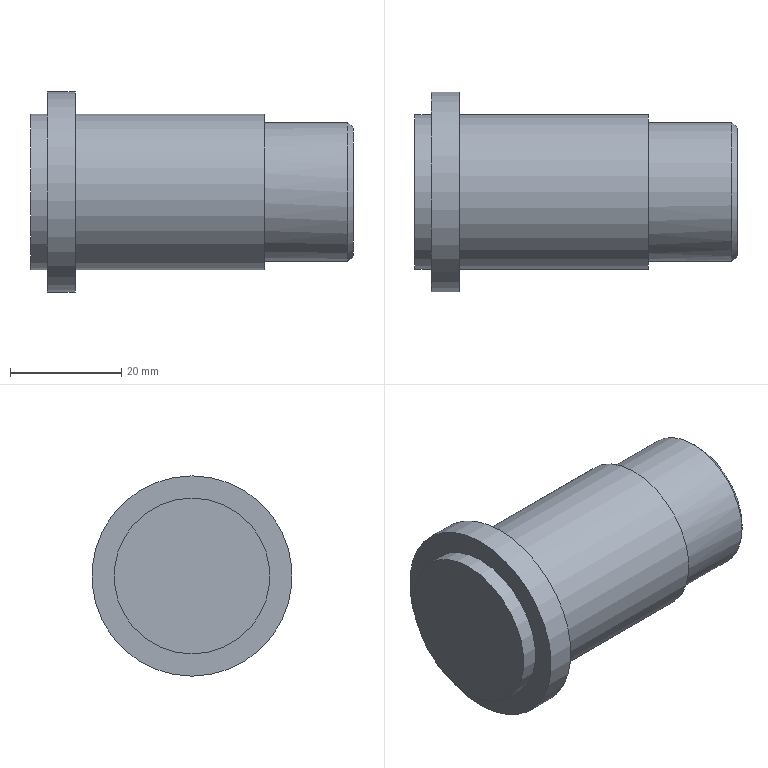Part | STEP file | zhou2 | 1 solid | 12 faces | box 58 x 36 x 36 mm | volume 34937 mm3 | cylinder 5 | plane 5 | cone 2 | commonest cylinder face diameters 28 x2 6.8 x1 25 x1 36 x1
STEP:
#1=CARTESIAN_POINT('',(0.,0.,0.));
#2=DIRECTION('',(0.,0.,1.));
#3=DIRECTION('',(1.,0.,0.));
#4=AXIS2_PLACEMENT_3D('',#1,#2,#3);
#5=CARTESIAN_POINT('',(8.,0.,14.));
#6=VERTEX_POINT('',#5);
#7=CARTESIAN_POINT('',(8.,0.,0.));
#8=DIRECTION('',(1.,0.,0.));
#9=DIRECTION('',(0.,0.,1.));
#10=AXIS2_PLACEMENT_3D('',#7,#8,#9);
#11=CIRCLE('',#10,14.);
#12=CARTESIAN_POINT('',(0.,0.,0.));
#13=DIRECTION('',(-1.,0.,0.));
#14=DIRECTION('',(0.,0.,1.));
#15=AXIS2_PLACEMENT_3D('',#12,#13,#14);
#16=CYLINDRICAL_SURFACE('',#15,14.);
#17=CARTESIAN_POINT('',(6.283,-8.));
#18=DIRECTION('',(-1.,0.));
#19=VECTOR('',#18,1.);
#20=LINE('',#17,#19);
#21=(GEOMETRIC_REPRESENTATION_CONTEXT(2)PARAMETRIC_REPRESENTATION_CONTEXT()REPRESENTATION_CONTEXT('',''));
#22=DEFINITIONAL_REPRESENTATION('',(#20),#21);
#23=PCURVE('',#16,#22);
#24=CARTESIAN_POINT('',(8.,18.,0.));
#25=DIRECTION('',(-1.,0.,0.));
#26=DIRECTION('',(0.,0.,1.));
#27=AXIS2_PLACEMENT_3D('',#24,#25,#26);
#28=PLANE('',#27);
#29=CARTESIAN_POINT('',(14.,-18.));
#30=CARTESIAN_POINT('',(14.,-42.249));
#31=CARTESIAN_POINT('',(-7.,-30.124));
#32=CARTESIAN_POINT('',(-28.,-18.));
#33=CARTESIAN_POINT('',(-7.,-5.876));
#34=CARTESIAN_POINT('',(14.,6.249));
#35=CARTESIAN_POINT('',(14.,-18.));
#36=(BOUNDED_CURVE()B_SPLINE_CURVE(2,(#29,#30,#31,#32,#33,#34,#35),.UNSPECIFIED.,.T.,.F.)B_SPLINE_CURVE_WITH_KNOTS((1,2,2,2,2,1),(-2.094,0.,2.094,4.189,6.283,8.378),.UNSPECIFIED.)CURVE()GEOMETRIC_REPRESENTATION_ITEM()RATIONAL_B_SPLINE_CURVE((1.,0.5,1.,0.5,1.,0.5,1.))REPRESENTATION_ITEM(''));
#37=(GEOMETRIC_REPRESENTATION_CONTEXT(2)PARAMETRIC_REPRESENTATION_CONTEXT()REPRESENTATION_CONTEXT('',''));
#38=DEFINITIONAL_REPRESENTATION('',(#36),#37);
#39=PCURVE('',#28,#38);
#40=SURFACE_CURVE('',#11,(#23,#39),.PCURVE_S1.);
#41=EDGE_CURVE('',#6,#6,#40,.T.);
#42=ORIENTED_EDGE('',*,*,#41,.T.);
#43=CARTESIAN_POINT('',(42.,0.,14.));
#44=VERTEX_POINT('',#43);
#45=CARTESIAN_POINT('',(42.,0.,14.));
#46=CARTESIAN_POINT('',(8.,0.,14.));
#47=B_SPLINE_CURVE_WITH_KNOTS('',1,(#45,#46),.UNSPECIFIED.,.F.,.F.,(2,2),(-42.,-8.),.PIECEWISE_BEZIER_KNOTS.);
#48=CARTESIAN_POINT('',(0.,0.));
#49=DIRECTION('',(0.,1.));
#50=VECTOR('',#49,1.);
#51=LINE('',#48,#50);
#52=(GEOMETRIC_REPRESENTATION_CONTEXT(2)PARAMETRIC_REPRESENTATION_CONTEXT()REPRESENTATION_CONTEXT('',''));
#53=DEFINITIONAL_REPRESENTATION('',(#51),#52);
#54=PCURVE('',#16,#53);
#55=CARTESIAN_POINT('',(6.283,0.));
#56=DIRECTION('',(0.,1.));
#57=VECTOR('',#56,1.);
#58=LINE('',#55,#57);
#59=(GEOMETRIC_REPRESENTATION_CONTEXT(2)PARAMETRIC_REPRESENTATION_CONTEXT()REPRESENTATION_CONTEXT('',''));
#60=DEFINITIONAL_REPRESENTATION('',(#58),#59);
#61=PCURVE('',#16,#60);
#62=SEAM_CURVE('',#47,(#54,#61),.PCURVE_S1.);
#63=EDGE_CURVE('',#44,#6,#62,.T.);
#64=ORIENTED_EDGE('',*,*,#63,.F.);
#65=CARTESIAN_POINT('',(42.,0.,0.));
#66=DIRECTION('',(-1.,0.,0.));
#67=DIRECTION('',(0.,0.,1.));
#68=AXIS2_PLACEMENT_3D('',#65,#66,#67);
#69=CIRCLE('',#68,14.);
#70=CARTESIAN_POINT('',(0.,-42.));
#71=DIRECTION('',(1.,0.));
#72=VECTOR('',#71,1.);
#73=LINE('',#70,#72);
#74=(GEOMETRIC_REPRESENTATION_CONTEXT(2)PARAMETRIC_REPRESENTATION_CONTEXT()REPRESENTATION_CONTEXT('',''));
#75=DEFINITIONAL_REPRESENTATION('',(#73),#74);
#76=PCURVE('',#16,#75);
#77=CARTESIAN_POINT('',(42.,14.,0.));
#78=DIRECTION('',(-1.,0.,0.));
#79=DIRECTION('',(0.,0.,1.));
#80=AXIS2_PLACEMENT_3D('',#77,#78,#79);
#81=PLANE('',#80);
#82=CARTESIAN_POINT('',(0.,-14.));
#83=DIRECTION('',(1.,0.));
#84=AXIS2_PLACEMENT_2D('',#82,#83);
#85=CIRCLE('',#84,14.);
#86=(GEOMETRIC_REPRESENTATION_CONTEXT(2)PARAMETRIC_REPRESENTATION_CONTEXT()REPRESENTATION_CONTEXT('',''));
#87=DEFINITIONAL_REPRESENTATION('',(#85),#86);
#88=PCURVE('',#81,#87);
#89=SURFACE_CURVE('',#69,(#76,#88),.PCURVE_S1.);
#90=EDGE_CURVE('',#44,#44,#89,.T.);
#91=ORIENTED_EDGE('',*,*,#90,.T.);
#92=ORIENTED_EDGE('',*,*,#63,.T.);
#93=EDGE_LOOP('',(#42,#64,#91,#92));
#94=FACE_BOUND('',#93,.T.);
#95=ADVANCED_FACE('',(#94),#16,.T.);
#96=ORIENTED_EDGE('',*,*,#41,.F.);
#97=EDGE_LOOP('',(#96));
#98=FACE_BOUND('',#97,.T.);
#99=CARTESIAN_POINT('',(8.,0.,18.));
#100=VERTEX_POINT('',#99);
#101=CARTESIAN_POINT('',(8.,0.,0.));
#102=DIRECTION('',(-1.,0.,0.));
#103=DIRECTION('',(0.,0.,1.));
#104=AXIS2_PLACEMENT_3D('',#101,#102,#103);
#105=CIRCLE('',#104,18.);
#106=CARTESIAN_POINT('',(0.,-18.));
#107=DIRECTION('',(1.,0.));
#108=AXIS2_PLACEMENT_2D('',#106,#107);
#109=CIRCLE('',#108,18.);
#110=(GEOMETRIC_REPRESENTATION_CONTEXT(2)PARAMETRIC_REPRESENTATION_CONTEXT()REPRESENTATION_CONTEXT('',''));
#111=DEFINITIONAL_REPRESENTATION('',(#109),#110);
#112=PCURVE('',#28,#111);
#113=CARTESIAN_POINT('',(0.,0.,0.));
#114=DIRECTION('',(-1.,0.,0.));
#115=DIRECTION('',(0.,0.,1.));
#116=AXIS2_PLACEMENT_3D('',#113,#114,#115);
#117=CYLINDRICAL_SURFACE('',#116,18.);
#118=CARTESIAN_POINT('',(0.,-8.));
#119=DIRECTION('',(1.,0.));
#120=VECTOR('',#119,1.);
#121=LINE('',#118,#120);
#122=(GEOMETRIC_REPRESENTATION_CONTEXT(2)PARAMETRIC_REPRESENTATION_CONTEXT()REPRESENTATION_CONTEXT('',''));
#123=DEFINITIONAL_REPRESENTATION('',(#121),#122);
#124=PCURVE('',#117,#123);
#125=SURFACE_CURVE('',#105,(#112,#124),.PCURVE_S1.);
#126=EDGE_CURVE('',#100,#100,#125,.T.);
#127=ORIENTED_EDGE('',*,*,#126,.F.);
#128=EDGE_LOOP('',(#127));
#129=FACE_BOUND('',#128,.T.);
#130=ADVANCED_FACE('',(#98,#129),#28,.F.);
#131=CARTESIAN_POINT('',(42.,0.,12.5));
#132=VERTEX_POINT('',#131);
#133=CARTESIAN_POINT('',(42.,0.,0.));
#134=DIRECTION('',(1.,0.,0.));
#135=DIRECTION('',(0.,0.,1.));
#136=AXIS2_PLACEMENT_3D('',#133,#134,#135);
#137=CIRCLE('',#136,12.5);
#138=CARTESIAN_POINT('',(12.5,-14.));
#139=CARTESIAN_POINT('',(12.5,-35.651));
#140=CARTESIAN_POINT('',(-6.25,-24.825));
#141=CARTESIAN_POINT('',(-25.,-14.));
#142=CARTESIAN_POINT('',(-6.25,-3.175));
#143=CARTESIAN_POINT('',(12.5,7.651));
#144=CARTESIAN_POINT('',(12.5,-14.));
#145=(BOUNDED_CURVE()B_SPLINE_CURVE(2,(#138,#139,#140,#141,#142,#143,#144),.UNSPECIFIED.,.T.,.F.)B_SPLINE_CURVE_WITH_KNOTS((1,2,2,2,2,1),(-2.094,0.,2.094,4.189,6.283,8.378),.UNSPECIFIED.)CURVE()GEOMETRIC_REPRESENTATION_ITEM()RATIONAL_B_SPLINE_CURVE((1.,0.5,1.,0.5,1.,0.5,1.))REPRESENTATION_ITEM(''));
#146=(GEOMETRIC_REPRESENTATION_CONTEXT(2)PARAMETRIC_REPRESENTATION_CONTEXT()REPRESENTATION_CONTEXT('',''));
#147=DEFINITIONAL_REPRESENTATION('',(#145),#146);
#148=PCURVE('',#81,#147);
#149=CARTESIAN_POINT('',(0.,0.,0.));
#150=DIRECTION('',(-1.,0.,0.));
#151=DIRECTION('',(0.,0.,1.));
#152=AXIS2_PLACEMENT_3D('',#149,#150,#151);
#153=CYLINDRICAL_SURFACE('',#152,12.5);
#154=CARTESIAN_POINT('',(6.283,-42.));
#155=DIRECTION('',(-1.,0.));
#156=VECTOR('',#155,1.);
#157=LINE('',#154,#156);
#158=(GEOMETRIC_REPRESENTATION_CONTEXT(2)PARAMETRIC_REPRESENTATION_CONTEXT()REPRESENTATION_CONTEXT('',''));
#159=DEFINITIONAL_REPRESENTATION('',(#157),#158);
#160=PCURVE('',#153,#159);
#161=SURFACE_CURVE('',#137,(#148,#160),.PCURVE_S1.);
#162=EDGE_CURVE('',#132,#132,#161,.T.);
#163=ORIENTED_EDGE('',*,*,#162,.F.);
#164=EDGE_LOOP('',(#163));
#165=FACE_BOUND('',#164,.T.);
#166=ORIENTED_EDGE('',*,*,#90,.F.);
#167=EDGE_LOOP('',(#166));
#168=FACE_BOUND('',#167,.T.);
#169=ADVANCED_FACE('',(#165,#168),#81,.F.);
#170=CARTESIAN_POINT('',(3.,0.,18.));
#171=VERTEX_POINT('',#170);
#172=CARTESIAN_POINT('',(3.,0.,0.));
#173=DIRECTION('',(1.,0.,0.));
#174=DIRECTION('',(0.,0.,1.));
#175=AXIS2_PLACEMENT_3D('',#172,#173,#174);
#176=CIRCLE('',#175,18.);
#177=CARTESIAN_POINT('',(6.283,-3.));
#178=DIRECTION('',(-1.,0.));
#179=VECTOR('',#178,1.);
#180=LINE('',#177,#179);
#181=(GEOMETRIC_REPRESENTATION_CONTEXT(2)PARAMETRIC_REPRESENTATION_CONTEXT()REPRESENTATION_CONTEXT('',''));
#182=DEFINITIONAL_REPRESENTATION('',(#180),#181);
#183=PCURVE('',#117,#182);
#184=CARTESIAN_POINT('',(3.,14.,0.));
#185=DIRECTION('',(1.,0.,0.));
#186=DIRECTION('',(0.,0.,-1.));
#187=AXIS2_PLACEMENT_3D('',#184,#185,#186);
#188=PLANE('',#187);
#189=CARTESIAN_POINT('',(0.,-14.));
#190=DIRECTION('',(-1.,0.));
#191=AXIS2_PLACEMENT_2D('',#189,#190);
#192=CIRCLE('',#191,18.);
#193=(GEOMETRIC_REPRESENTATION_CONTEXT(2)PARAMETRIC_REPRESENTATION_CONTEXT()REPRESENTATION_CONTEXT('',''));
#194=DEFINITIONAL_REPRESENTATION('',(#192),#193);
#195=PCURVE('',#188,#194);
#196=SURFACE_CURVE('',#176,(#183,#195),.PCURVE_S1.);
#197=EDGE_CURVE('',#171,#171,#196,.T.);
#198=ORIENTED_EDGE('',*,*,#197,.T.);
#199=CARTESIAN_POINT('',(8.,0.,18.));
#200=CARTESIAN_POINT('',(3.,0.,18.));
#201=B_SPLINE_CURVE_WITH_KNOTS('',1,(#199,#200),.UNSPECIFIED.,.F.,.F.,(2,2),(-8.,-3.),.PIECEWISE_BEZIER_KNOTS.);
#202=CARTESIAN_POINT('',(0.,0.));
#203=DIRECTION('',(0.,1.));
#204=VECTOR('',#203,1.);
#205=LINE('',#202,#204);
#206=(GEOMETRIC_REPRESENTATION_CONTEXT(2)PARAMETRIC_REPRESENTATION_CONTEXT()REPRESENTATION_CONTEXT('',''));
#207=DEFINITIONAL_REPRESENTATION('',(#205),#206);
#208=PCURVE('',#117,#207);
#209=CARTESIAN_POINT('',(6.283,0.));
#210=DIRECTION('',(0.,1.));
#211=VECTOR('',#210,1.);
#212=LINE('',#209,#211);
#213=(GEOMETRIC_REPRESENTATION_CONTEXT(2)PARAMETRIC_REPRESENTATION_CONTEXT()REPRESENTATION_CONTEXT('',''));
#214=DEFINITIONAL_REPRESENTATION('',(#212),#213);
#215=PCURVE('',#117,#214);
#216=SEAM_CURVE('',#201,(#208,#215),.PCURVE_S1.);
#217=EDGE_CURVE('',#100,#171,#216,.T.);
#218=ORIENTED_EDGE('',*,*,#217,.F.);
#219=ORIENTED_EDGE('',*,*,#126,.T.);
#220=ORIENTED_EDGE('',*,*,#217,.T.);
#221=EDGE_LOOP('',(#198,#218,#219,#220));
#222=FACE_BOUND('',#221,.T.);
#223=ADVANCED_FACE('',(#222),#117,.T.);
#224=ORIENTED_EDGE('',*,*,#162,.T.);
#225=CARTESIAN_POINT('',(57.,0.,12.5));
#226=VERTEX_POINT('',#225);
#227=CARTESIAN_POINT('',(57.,0.,12.5));
#228=CARTESIAN_POINT('',(42.,0.,12.5));
#229=B_SPLINE_CURVE_WITH_KNOTS('',1,(#227,#228),.UNSPECIFIED.,.F.,.F.,(2,2),(-57.,-42.),.PIECEWISE_BEZIER_KNOTS.);
#230=CARTESIAN_POINT('',(0.,0.));
#231=DIRECTION('',(0.,1.));
#232=VECTOR('',#231,1.);
#233=LINE('',#230,#232);
#234=(GEOMETRIC_REPRESENTATION_CONTEXT(2)PARAMETRIC_REPRESENTATION_CONTEXT()REPRESENTATION_CONTEXT('',''));
#235=DEFINITIONAL_REPRESENTATION('',(#233),#234);
#236=PCURVE('',#153,#235);
#237=CARTESIAN_POINT('',(6.283,0.));
#238=DIRECTION('',(0.,1.));
#239=VECTOR('',#238,1.);
#240=LINE('',#237,#239);
#241=(GEOMETRIC_REPRESENTATION_CONTEXT(2)PARAMETRIC_REPRESENTATION_CONTEXT()REPRESENTATION_CONTEXT('',''));
#242=DEFINITIONAL_REPRESENTATION('',(#240),#241);
#243=PCURVE('',#153,#242);
#244=SEAM_CURVE('',#229,(#236,#243),.PCURVE_S1.);
#245=EDGE_CURVE('',#226,#132,#244,.T.);
#246=ORIENTED_EDGE('',*,*,#245,.F.);
#247=CARTESIAN_POINT('',(57.,-12.5,0.));
#248=VERTEX_POINT('',#247);
#249=CARTESIAN_POINT('',(57.,0.,0.));
#250=DIRECTION('',(-1.,0.,0.));
#251=DIRECTION('',(0.,0.,1.));
#252=AXIS2_PLACEMENT_3D('',#249,#250,#251);
#253=CIRCLE('',#252,12.5);
#254=CARTESIAN_POINT('',(0.,-57.));
#255=DIRECTION('',(1.,0.));
#256=VECTOR('',#255,1.);
#257=LINE('',#254,#256);
#258=(GEOMETRIC_REPRESENTATION_CONTEXT(2)PARAMETRIC_REPRESENTATION_CONTEXT()REPRESENTATION_CONTEXT('',''));
#259=DEFINITIONAL_REPRESENTATION('',(#257),#258);
#260=PCURVE('',#153,#259);
#261=CARTESIAN_POINT('',(57.,0.,0.));
#262=DIRECTION('',(-1.,0.,0.));
#263=DIRECTION('',(0.,-1.,0.));
#264=AXIS2_PLACEMENT_3D('',#261,#262,#263);
#265=CONICAL_SURFACE('',#264,12.5,0.7854);
#266=CARTESIAN_POINT('',(1.571,0.));
#267=DIRECTION('',(1.,0.));
#268=VECTOR('',#267,1.);
#269=LINE('',#266,#268);
#270=(GEOMETRIC_REPRESENTATION_CONTEXT(2)PARAMETRIC_REPRESENTATION_CONTEXT()REPRESENTATION_CONTEXT('',''));
#271=DEFINITIONAL_REPRESENTATION('',(#269),#270);
#272=PCURVE('',#265,#271);
#273=SURFACE_CURVE('',#253,(#260,#272),.PCURVE_S1.);
#274=EDGE_CURVE('',#226,#248,#273,.T.);
#275=ORIENTED_EDGE('',*,*,#274,.T.);
#276=CARTESIAN_POINT('',(57.,0.,0.));
#277=DIRECTION('',(-1.,0.,0.));
#278=DIRECTION('',(0.,0.,1.));
#279=AXIS2_PLACEMENT_3D('',#276,#277,#278);
#280=CIRCLE('',#279,12.5);
#281=CARTESIAN_POINT('',(0.,-57.));
#282=DIRECTION('',(1.,0.));
#283=VECTOR('',#282,1.);
#284=LINE('',#281,#283);
#285=(GEOMETRIC_REPRESENTATION_CONTEXT(2)PARAMETRIC_REPRESENTATION_CONTEXT()REPRESENTATION_CONTEXT('',''));
#286=DEFINITIONAL_REPRESENTATION('',(#284),#285);
#287=PCURVE('',#153,#286);
#288=CARTESIAN_POINT('',(-4.712,0.));
#289=DIRECTION('',(1.,0.));
#290=VECTOR('',#289,1.);
#291=LINE('',#288,#290);
#292=(GEOMETRIC_REPRESENTATION_CONTEXT(2)PARAMETRIC_REPRESENTATION_CONTEXT()REPRESENTATION_CONTEXT('',''));
#293=DEFINITIONAL_REPRESENTATION('',(#291),#292);
#294=PCURVE('',#265,#293);
#295=SURFACE_CURVE('',#280,(#287,#294),.PCURVE_S1.);
#296=EDGE_CURVE('',#248,#226,#295,.T.);
#297=ORIENTED_EDGE('',*,*,#296,.T.);
#298=ORIENTED_EDGE('',*,*,#245,.T.);
#299=EDGE_LOOP('',(#224,#246,#275,#297,#298));
#300=FACE_BOUND('',#299,.T.);
#301=ADVANCED_FACE('',(#300),#153,.T.);
#302=ORIENTED_EDGE('',*,*,#197,.F.);
#303=EDGE_LOOP('',(#302));
#304=FACE_BOUND('',#303,.T.);
#305=CARTESIAN_POINT('',(3.,0.,14.));
#306=VERTEX_POINT('',#305);
#307=CARTESIAN_POINT('',(3.,0.,0.));
#308=DIRECTION('',(-1.,0.,0.));
#309=DIRECTION('',(0.,0.,1.));
#310=AXIS2_PLACEMENT_3D('',#307,#308,#309);
#311=CIRCLE('',#310,14.);
#312=CARTESIAN_POINT('',(-14.,-14.));
#313=CARTESIAN_POINT('',(-14.,10.249));
#314=CARTESIAN_POINT('',(7.,-1.876));
#315=CARTESIAN_POINT('',(28.,-14.));
#316=CARTESIAN_POINT('',(7.,-26.124));
#317=CARTESIAN_POINT('',(-14.,-38.249));
#318=CARTESIAN_POINT('',(-14.,-14.));
#319=(BOUNDED_CURVE()B_SPLINE_CURVE(2,(#312,#313,#314,#315,#316,#317,#318),.UNSPECIFIED.,.T.,.F.)B_SPLINE_CURVE_WITH_KNOTS((1,2,2,2,2,1),(-2.094,0.,2.094,4.189,6.283,8.378),.UNSPECIFIED.)CURVE()GEOMETRIC_REPRESENTATION_ITEM()RATIONAL_B_SPLINE_CURVE((1.,0.5,1.,0.5,1.,0.5,1.))REPRESENTATION_ITEM(''));
#320=(GEOMETRIC_REPRESENTATION_CONTEXT(2)PARAMETRIC_REPRESENTATION_CONTEXT()REPRESENTATION_CONTEXT('',''));
#321=DEFINITIONAL_REPRESENTATION('',(#319),#320);
#322=PCURVE('',#188,#321);
#323=CARTESIAN_POINT('',(0.,0.,0.));
#324=DIRECTION('',(-1.,0.,0.));
#325=DIRECTION('',(0.,0.,1.));
#326=AXIS2_PLACEMENT_3D('',#323,#324,#325);
#327=CYLINDRICAL_SURFACE('',#326,14.);
#328=CARTESIAN_POINT('',(0.,-3.));
#329=DIRECTION('',(1.,0.));
#330=VECTOR('',#329,1.);
#331=LINE('',#328,#330);
#332=(GEOMETRIC_REPRESENTATION_CONTEXT(2)PARAMETRIC_REPRESENTATION_CONTEXT()REPRESENTATION_CONTEXT('',''));
#333=DEFINITIONAL_REPRESENTATION('',(#331),#332);
#334=PCURVE('',#327,#333);
#335=SURFACE_CURVE('',#311,(#322,#334),.PCURVE_S1.);
#336=EDGE_CURVE('',#306,#306,#335,.T.);
#337=ORIENTED_EDGE('',*,*,#336,.F.);
#338=EDGE_LOOP('',(#337));
#339=FACE_BOUND('',#338,.T.);
#340=ADVANCED_FACE('',(#304,#339),#188,.F.);
#341=ORIENTED_EDGE('',*,*,#296,.F.);
#342=CARTESIAN_POINT('',(58.,-11.5,0.));
#343=VERTEX_POINT('',#342);
#344=CARTESIAN_POINT('',(58.,-11.5,0.));
#345=CARTESIAN_POINT('',(57.,-12.5,0.));
#346=B_SPLINE_CURVE_WITH_KNOTS('',1,(#344,#345),.UNSPECIFIED.,.F.,.F.,(2,2),(-1.414,0.),.PIECEWISE_BEZIER_KNOTS.);
#347=CARTESIAN_POINT('',(0.,0.));
#348=DIRECTION('',(0.,1.));
#349=VECTOR('',#348,1.);
#350=LINE('',#347,#349);
#351=(GEOMETRIC_REPRESENTATION_CONTEXT(2)PARAMETRIC_REPRESENTATION_CONTEXT()REPRESENTATION_CONTEXT('',''));
#352=DEFINITIONAL_REPRESENTATION('',(#350),#351);
#353=PCURVE('',#265,#352);
#354=CARTESIAN_POINT('',(6.283,0.));
#355=DIRECTION('',(0.,1.));
#356=VECTOR('',#355,1.);
#357=LINE('',#354,#356);
#358=(GEOMETRIC_REPRESENTATION_CONTEXT(2)PARAMETRIC_REPRESENTATION_CONTEXT()REPRESENTATION_CONTEXT('',''));
#359=DEFINITIONAL_REPRESENTATION('',(#357),#358);
#360=PCURVE('',#265,#359);
#361=SEAM_CURVE('',#346,(#353,#360),.PCURVE_S1.);
#362=EDGE_CURVE('',#343,#248,#361,.T.);
#363=ORIENTED_EDGE('',*,*,#362,.F.);
#364=CARTESIAN_POINT('',(58.,0.,0.));
#365=DIRECTION('',(-1.,0.,0.));
#366=DIRECTION('',(0.,-1.,0.));
#367=AXIS2_PLACEMENT_3D('',#364,#365,#366);
#368=CIRCLE('',#367,11.5);
#369=CARTESIAN_POINT('',(0.,-1.));
#370=DIRECTION('',(1.,0.));
#371=VECTOR('',#370,1.);
#372=LINE('',#369,#371);
#373=(GEOMETRIC_REPRESENTATION_CONTEXT(2)PARAMETRIC_REPRESENTATION_CONTEXT()REPRESENTATION_CONTEXT('',''));
#374=DEFINITIONAL_REPRESENTATION('',(#372),#373);
#375=PCURVE('',#265,#374);
#376=CARTESIAN_POINT('',(58.,12.5,0.));
#377=DIRECTION('',(-1.,0.,0.));
#378=DIRECTION('',(0.,0.,1.));
#379=AXIS2_PLACEMENT_3D('',#376,#377,#378);
#380=PLANE('',#379);
#381=CARTESIAN_POINT('',(0.,-12.5));
#382=DIRECTION('',(0.,-1.));
#383=AXIS2_PLACEMENT_2D('',#381,#382);
#384=CIRCLE('',#383,11.5);
#385=(GEOMETRIC_REPRESENTATION_CONTEXT(2)PARAMETRIC_REPRESENTATION_CONTEXT()REPRESENTATION_CONTEXT('',''));
#386=DEFINITIONAL_REPRESENTATION('',(#384),#385);
#387=PCURVE('',#380,#386);
#388=SURFACE_CURVE('',#368,(#375,#387),.PCURVE_S1.);
#389=EDGE_CURVE('',#343,#343,#388,.T.);
#390=ORIENTED_EDGE('',*,*,#389,.T.);
#391=ORIENTED_EDGE('',*,*,#362,.T.);
#392=ORIENTED_EDGE('',*,*,#274,.F.);
#393=EDGE_LOOP('',(#341,#363,#390,#391,#392));
#394=FACE_BOUND('',#393,.T.);
#395=ADVANCED_FACE('',(#394),#265,.T.);
#396=CARTESIAN_POINT('',(0.,0.,14.));
#397=VERTEX_POINT('',#396);
#398=CARTESIAN_POINT('',(0.,0.,0.));
#399=DIRECTION('',(1.,0.,0.));
#400=DIRECTION('',(0.,0.,1.));
#401=AXIS2_PLACEMENT_3D('',#398,#399,#400);
#402=CIRCLE('',#401,14.);
#403=CARTESIAN_POINT('',(6.283,0.));
#404=DIRECTION('',(-1.,0.));
#405=VECTOR('',#404,1.);
#406=LINE('',#403,#405);
#407=(GEOMETRIC_REPRESENTATION_CONTEXT(2)PARAMETRIC_REPRESENTATION_CONTEXT()REPRESENTATION_CONTEXT('',''));
#408=DEFINITIONAL_REPRESENTATION('',(#406),#407);
#409=PCURVE('',#327,#408);
#410=CARTESIAN_POINT('',(0.,0.,0.));
#411=DIRECTION('',(1.,0.,0.));
#412=DIRECTION('',(0.,0.,-1.));
#413=AXIS2_PLACEMENT_3D('',#410,#411,#412);
#414=PLANE('',#413);
#415=CARTESIAN_POINT('',(0.,0.));
#416=DIRECTION('',(-1.,0.));
#417=AXIS2_PLACEMENT_2D('',#415,#416);
#418=CIRCLE('',#417,14.);
#419=(GEOMETRIC_REPRESENTATION_CONTEXT(2)PARAMETRIC_REPRESENTATION_CONTEXT()REPRESENTATION_CONTEXT('',''));
#420=DEFINITIONAL_REPRESENTATION('',(#418),#419);
#421=PCURVE('',#414,#420);
#422=SURFACE_CURVE('',#402,(#409,#421),.PCURVE_S1.);
#423=EDGE_CURVE('',#397,#397,#422,.T.);
#424=ORIENTED_EDGE('',*,*,#423,.T.);
#425=CARTESIAN_POINT('',(3.,0.,14.));
#426=CARTESIAN_POINT('',(0.,0.,14.));
#427=B_SPLINE_CURVE_WITH_KNOTS('',1,(#425,#426),.UNSPECIFIED.,.F.,.F.,(2,2),(-3.,0.),.PIECEWISE_BEZIER_KNOTS.);
#428=CARTESIAN_POINT('',(0.,0.));
#429=DIRECTION('',(0.,1.));
#430=VECTOR('',#429,1.);
#431=LINE('',#428,#430);
#432=(GEOMETRIC_REPRESENTATION_CONTEXT(2)PARAMETRIC_REPRESENTATION_CONTEXT()REPRESENTATION_CONTEXT('',''));
#433=DEFINITIONAL_REPRESENTATION('',(#431),#432);
#434=PCURVE('',#327,#433);
#435=CARTESIAN_POINT('',(6.283,0.));
#436=DIRECTION('',(0.,1.));
#437=VECTOR('',#436,1.);
#438=LINE('',#435,#437);
#439=(GEOMETRIC_REPRESENTATION_CONTEXT(2)PARAMETRIC_REPRESENTATION_CONTEXT()REPRESENTATION_CONTEXT('',''));
#440=DEFINITIONAL_REPRESENTATION('',(#438),#439);
#441=PCURVE('',#327,#440);
#442=SEAM_CURVE('',#427,(#434,#441),.PCURVE_S1.);
#443=EDGE_CURVE('',#306,#397,#442,.T.);
#444=ORIENTED_EDGE('',*,*,#443,.F.);
#445=ORIENTED_EDGE('',*,*,#336,.T.);
#446=ORIENTED_EDGE('',*,*,#443,.T.);
#447=EDGE_LOOP('',(#424,#444,#445,#446));
#448=FACE_BOUND('',#447,.T.);
#449=ADVANCED_FACE('',(#448),#327,.T.);
#450=ORIENTED_EDGE('',*,*,#389,.F.);
#451=EDGE_LOOP('',(#450));
#452=FACE_BOUND('',#451,.T.);
#453=CARTESIAN_POINT('',(58.,0.,-3.4));
#454=VERTEX_POINT('',#453);
#455=CARTESIAN_POINT('',(58.,0.,0.));
#456=DIRECTION('',(1.,0.,0.));
#457=DIRECTION('',(0.,0.,-1.));
#458=AXIS2_PLACEMENT_3D('',#455,#456,#457);
#459=CIRCLE('',#458,3.4);
#460=CARTESIAN_POINT('',(-3.4,-12.5));
#461=CARTESIAN_POINT('',(-3.4,-6.611));
#462=CARTESIAN_POINT('',(1.7,-9.556));
#463=CARTESIAN_POINT('',(6.8,-12.5));
#464=CARTESIAN_POINT('',(1.7,-15.444));
#465=CARTESIAN_POINT('',(-3.4,-18.389));
#466=CARTESIAN_POINT('',(-3.4,-12.5));
#467=(BOUNDED_CURVE()B_SPLINE_CURVE(2,(#460,#461,#462,#463,#464,#465,#466),.UNSPECIFIED.,.T.,.F.)B_SPLINE_CURVE_WITH_KNOTS((1,2,2,2,2,1),(-2.094,0.,2.094,4.189,6.283,8.378),.UNSPECIFIED.)CURVE()GEOMETRIC_REPRESENTATION_ITEM()RATIONAL_B_SPLINE_CURVE((1.,0.5,1.,0.5,1.,0.5,1.))REPRESENTATION_ITEM(''));
#468=(GEOMETRIC_REPRESENTATION_CONTEXT(2)PARAMETRIC_REPRESENTATION_CONTEXT()REPRESENTATION_CONTEXT('',''));
#469=DEFINITIONAL_REPRESENTATION('',(#467),#468);
#470=PCURVE('',#380,#469);
#471=CARTESIAN_POINT('',(58.,0.,0.));
#472=DIRECTION('',(1.,0.,0.));
#473=DIRECTION('',(0.,0.,-1.));
#474=AXIS2_PLACEMENT_3D('',#471,#472,#473);
#475=CYLINDRICAL_SURFACE('',#474,3.4);
#476=CARTESIAN_POINT('',(0.,0.));
#477=DIRECTION('',(1.,0.));
#478=VECTOR('',#477,1.);
#479=LINE('',#476,#478);
#480=(GEOMETRIC_REPRESENTATION_CONTEXT(2)PARAMETRIC_REPRESENTATION_CONTEXT()REPRESENTATION_CONTEXT('',''));
#481=DEFINITIONAL_REPRESENTATION('',(#479),#480);
#482=PCURVE('',#475,#481);
#483=SURFACE_CURVE('',#459,(#470,#482),.PCURVE_S1.);
#484=EDGE_CURVE('',#454,#454,#483,.T.);
#485=ORIENTED_EDGE('',*,*,#484,.F.);
#486=EDGE_LOOP('',(#485));
#487=FACE_BOUND('',#486,.T.);
#488=ADVANCED_FACE('',(#452,#487),#380,.F.);
#489=ORIENTED_EDGE('',*,*,#423,.F.);
#490=EDGE_LOOP('',(#489));
#491=FACE_BOUND('',#490,.T.);
#492=ADVANCED_FACE('',(#491),#414,.F.);
#493=CARTESIAN_POINT('',(38.,0.,-3.4));
#494=VERTEX_POINT('',#493);
#495=CARTESIAN_POINT('',(38.,0.,0.));
#496=DIRECTION('',(1.,0.,0.));
#497=DIRECTION('',(0.,0.,-1.));
#498=AXIS2_PLACEMENT_3D('',#495,#496,#497);
#499=CIRCLE('',#498,3.4);
#500=CARTESIAN_POINT('',(0.,-20.));
#501=DIRECTION('',(1.,0.));
#502=VECTOR('',#501,1.);
#503=LINE('',#500,#502);
#504=(GEOMETRIC_REPRESENTATION_CONTEXT(2)PARAMETRIC_REPRESENTATION_CONTEXT()REPRESENTATION_CONTEXT('',''));
#505=DEFINITIONAL_REPRESENTATION('',(#503),#504);
#506=PCURVE('',#475,#505);
#507=CARTESIAN_POINT('',(38.,0.,0.));
#508=DIRECTION('',(1.,0.,0.));
#509=DIRECTION('',(0.,0.,-1.));
#510=AXIS2_PLACEMENT_3D('',#507,#508,#509);
#511=CONICAL_SURFACE('',#510,3.4,1.03);
#512=CARTESIAN_POINT('',(0.,0.));
#513=DIRECTION('',(1.,0.));
#514=VECTOR('',#513,1.);
#515=LINE('',#512,#514);
#516=(GEOMETRIC_REPRESENTATION_CONTEXT(2)PARAMETRIC_REPRESENTATION_CONTEXT()REPRESENTATION_CONTEXT('',''));
#517=DEFINITIONAL_REPRESENTATION('',(#515),#516);
#518=PCURVE('',#511,#517);
#519=SURFACE_CURVE('',#499,(#506,#518),.PCURVE_S1.);
#520=EDGE_CURVE('',#494,#494,#519,.T.);
#521=ORIENTED_EDGE('',*,*,#520,.T.);
#522=CARTESIAN_POINT('',(38.,0.,-3.4));
#523=CARTESIAN_POINT('',(58.,0.,-3.4));
#524=B_SPLINE_CURVE_WITH_KNOTS('',1,(#522,#523),.UNSPECIFIED.,.F.,.F.,(2,2),(-20.,0.),.PIECEWISE_BEZIER_KNOTS.);
#525=CARTESIAN_POINT('',(6.283,0.));
#526=DIRECTION('',(0.,1.));
#527=VECTOR('',#526,1.);
#528=LINE('',#525,#527);
#529=(GEOMETRIC_REPRESENTATION_CONTEXT(2)PARAMETRIC_REPRESENTATION_CONTEXT()REPRESENTATION_CONTEXT('',''));
#530=DEFINITIONAL_REPRESENTATION('',(#528),#529);
#531=PCURVE('',#475,#530);
#532=CARTESIAN_POINT('',(0.,0.));
#533=DIRECTION('',(0.,1.));
#534=VECTOR('',#533,1.);
#535=LINE('',#532,#534);
#536=(GEOMETRIC_REPRESENTATION_CONTEXT(2)PARAMETRIC_REPRESENTATION_CONTEXT()REPRESENTATION_CONTEXT('',''));
#537=DEFINITIONAL_REPRESENTATION('',(#535),#536);
#538=PCURVE('',#475,#537);
#539=SEAM_CURVE('',#524,(#531,#538),.PCURVE_S1.);
#540=EDGE_CURVE('',#494,#454,#539,.T.);
#541=ORIENTED_EDGE('',*,*,#540,.T.);
#542=ORIENTED_EDGE('',*,*,#484,.F.);
#543=ORIENTED_EDGE('',*,*,#540,.F.);
#544=EDGE_LOOP('',(#521,#541,#542,#543));
#545=FACE_BOUND('',#544,.F.);
#546=ADVANCED_FACE('',(#545),#475,.F.);
#547=ORIENTED_EDGE('',*,*,#520,.F.);
#548=CARTESIAN_POINT('',(35.957,0.,0.));
#549=VERTEX_POINT('',#548);
#550=CARTESIAN_POINT('',(35.957,0.,0.));
#551=CARTESIAN_POINT('',(38.,0.,-3.4));
#552=B_SPLINE_CURVE_WITH_KNOTS('',1,(#550,#551),.UNSPECIFIED.,.F.,.F.,(2,2),(-3.967,0.),.PIECEWISE_BEZIER_KNOTS.);
#553=CARTESIAN_POINT('',(0.,0.));
#554=DIRECTION('',(0.,1.));
#555=VECTOR('',#554,1.);
#556=LINE('',#553,#555);
#557=(GEOMETRIC_REPRESENTATION_CONTEXT(2)PARAMETRIC_REPRESENTATION_CONTEXT()REPRESENTATION_CONTEXT('',''));
#558=DEFINITIONAL_REPRESENTATION('',(#556),#557);
#559=PCURVE('',#511,#558);
#560=CARTESIAN_POINT('',(6.283,0.));
#561=DIRECTION('',(0.,1.));
#562=VECTOR('',#561,1.);
#563=LINE('',#560,#562);
#564=(GEOMETRIC_REPRESENTATION_CONTEXT(2)PARAMETRIC_REPRESENTATION_CONTEXT()REPRESENTATION_CONTEXT('',''));
#565=DEFINITIONAL_REPRESENTATION('',(#563),#564);
#566=PCURVE('',#511,#565);
#567=SEAM_CURVE('',#552,(#559,#566),.PCURVE_S1.);
#568=EDGE_CURVE('',#549,#494,#567,.T.);
#569=ORIENTED_EDGE('',*,*,#568,.F.);
#570=ORIENTED_EDGE('',*,*,#568,.T.);
#571=EDGE_LOOP('',(#547,#569,#570));
#572=FACE_BOUND('',#571,.F.);
#573=ADVANCED_FACE('',(#572),#511,.F.);
#574=CLOSED_SHELL('',(#95,#130,#169,#223,#301,#340,#395,#449,#488,#492,#546,#573));
#575=MANIFOLD_SOLID_BREP('',#574);
#576=(LENGTH_UNIT()NAMED_UNIT(*)SI_UNIT(.MILLI.,.METRE.));
#577=UNCERTAINTY_MEASURE_WITH_UNIT(LENGTH_MEASURE(0.00001),#576,'','');
#578=(NAMED_UNIT(*)PLANE_ANGLE_UNIT()SI_UNIT($,.RADIAN.));
#579=(NAMED_UNIT(*)SI_UNIT($,.STERADIAN.)SOLID_ANGLE_UNIT());
#580=(GEOMETRIC_REPRESENTATION_CONTEXT(3)GLOBAL_UNCERTAINTY_ASSIGNED_CONTEXT((#577))GLOBAL_UNIT_ASSIGNED_CONTEXT((#576,#578,#579))REPRESENTATION_CONTEXT('',''));
#581=ADVANCED_BREP_SHAPE_REPRESENTATION('',(#4,#575),#580);